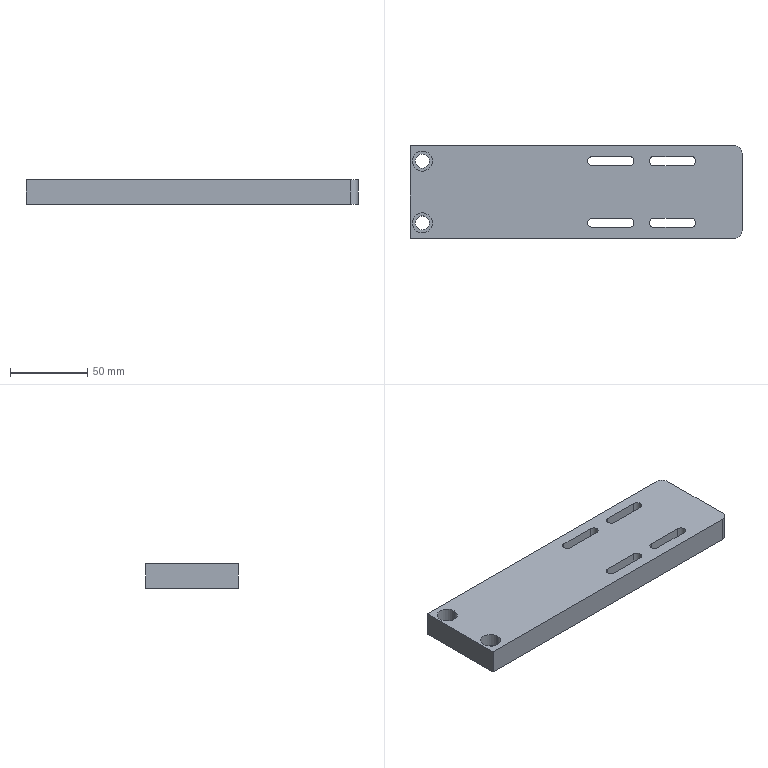NC program | Mastercam | posted with a generic post | part box 215 x 60 x 16 mm
Lines 24 to 1423 of 6620:
N230 T10 M6
N240 G0 G90 G17 G54 X-115.323 Y-40.256 A0. S7000 M3
N250 G43 H10 Z20. M8
N260 Z1.
N270 G1 Z-16.75 F600.
N280 X-115.624 Y-39.448 Z-16.868 F3000.
N290 G3 X-116.142 Y-38.642 Z-17. I-2.109 J-.785
N300 G1 X-116.424 Y-38.172
N310 X-116.706 Y-37.594
N320 X-116.919 Y-37.071
N330 X-117.071 Y-36.601
N340 X-117.179 Y-36.179
N350 X-117.254 Y-35.799
N360 X-117.347 Y-35.146
N370 X-117.4 Y-34.565
N380 X-117.429 Y-34.035
N390 X-117.443 Y-33.54
N400 X-117.45 Y-33.069
N410 X-117.451 Y-32.614
N420 X-117.449 Y-32.17
N430 X-117.444 Y-31.733
N440 X-117.439 Y-31.299
N450 X-117.433 Y-30.868
N460 X-117.426 Y-30.438
N470 X-117.419 Y-30.009
N480 X-117.412 Y-29.58
N490 X-117.405 Y-29.151
N500 X-117.397 Y-28.721
N510 X-117.39 Y-28.292
N520 X-117.382 Y-27.863
N530 X-117.374 Y-27.433
N540 X-117.367 Y-27.003
N550 X-117.359 Y-26.573
N560 X-117.352 Y-26.142
N570 X-117.344 Y-25.712
N580 X-117.336 Y-25.281
N590 X-117.329 Y-24.849
N600 X-117.321 Y-24.418
N610 X-117.313 Y-23.986
N620 X-117.305 Y-23.554
N630 X-117.298 Y-23.122
N640 X-117.29 Y-22.689
N650 X-117.282 Y-22.256
N660 X-117.275 Y-21.824
N670 X-117.267 Y-21.39
N680 X-117.259 Y-20.957
N690 X-117.252 Y-20.524
N700 X-117.244 Y-20.09
N710 X-117.236 Y-19.656
N720 X-117.228 Y-19.222
N730 X-117.221 Y-18.788
N740 X-117.213 Y-18.353
N750 X-117.205 Y-17.919
N760 X-117.197 Y-17.484
N770 X-117.19 Y-17.049
N780 X-117.182 Y-16.614
N790 X-117.174 Y-16.179
N800 X-117.166 Y-15.743
N810 X-117.159 Y-15.308
N820 X-117.151 Y-14.872
N830 X-117.143 Y-14.436
N840 X-117.135 Y-14.
N850 X-117.128 Y-13.564
N860 X-117.12 Y-13.128
N870 X-117.112 Y-12.692
N880 X-117.104 Y-12.255
N890 X-117.097 Y-11.819
N900 X-117.089 Y-11.382
N910 X-117.081 Y-10.945
N920 X-117.073 Y-10.508
N930 X-117.065 Y-10.071
N940 X-117.058 Y-9.634
N950 X-117.05 Y-9.197
N960 X-117.042 Y-8.759
N970 X-117.034 Y-8.322
N980 X-117.026 Y-7.884
N990 X-117.019 Y-7.446
N1000 X-117.011 Y-7.008
N1010 X-117.003 Y-6.571
N1020 X-116.995 Y-6.133
N1030 X-116.987 Y-5.694
N1040 X-116.98 Y-5.256
N1050 X-116.972 Y-4.818
N1060 X-116.964 Y-4.379
N1070 X-116.956 Y-3.941
N1080 X-116.948 Y-3.502
N1090 X-116.941 Y-3.064
N1100 X-116.933 Y-2.625
N1110 X-116.925 Y-2.186
N1120 X-116.917 Y-1.747
N1130 X-116.909 Y-1.308
N1140 X-116.902 Y-.869
N1150 X-116.894 Y-.43
N1160 X-116.886 Y.009
N1170 X-116.878 Y.449
N1180 X-116.87 Y.888
N1190 X-116.862 Y1.328
N1200 X-116.855 Y1.767
N1210 X-116.847 Y2.207
N1220 X-116.839 Y2.647
N1230 X-116.831 Y3.086
N1240 X-116.823 Y3.526
N1250 X-116.815 Y3.966
N1260 X-116.808 Y4.406
N1270 X-116.8 Y4.846
N1280 X-116.792 Y5.286
N1290 X-116.784 Y5.727
N1300 X-116.776 Y6.167
N1310 X-116.768 Y6.607
N1320 X-116.761 Y7.048
N1330 X-116.753 Y7.488
N1340 X-116.745 Y7.929
N1350 X-116.737 Y8.369
N1360 X-116.729 Y8.81
N1370 X-116.721 Y9.251
N1380 X-116.714 Y9.692
N1390 X-116.706 Y10.132
N1400 X-116.698 Y10.573
N1410 X-116.69 Y11.014
N1420 X-116.682 Y11.455
N1430 X-116.674 Y11.896
N1440 X-116.666 Y12.338
N1450 X-116.659 Y12.779
N1460 X-116.651 Y13.22
N1470 X-116.643 Y13.661
N1480 X-116.635 Y14.103
N1490 X-116.627 Y14.544
N1500 X-116.619 Y14.986
N1510 X-116.611 Y15.427
N1520 X-116.604 Y15.869
N1530 X-116.596 Y16.31
N1540 X-116.588 Y16.752
N1550 X-116.58 Y17.194
N1560 X-116.572 Y17.636
N1570 X-116.564 Y18.078
N1580 X-116.556 Y18.519
N1590 X-116.549 Y18.961
N1600 X-116.541 Y19.403
N1610 X-116.533 Y19.845
N1620 X-116.525 Y20.288
N1630 X-116.517 Y20.73
N1640 X-116.509 Y21.172
N1650 X-116.501 Y21.614
N1660 X-116.493 Y22.056
N1670 X-116.486 Y22.499
N1680 X-116.478 Y22.941
N1690 X-116.47 Y23.384
N1700 X-116.462 Y23.826
N1710 X-116.454 Y24.269
N1720 X-116.446 Y24.711
N1730 X-116.438 Y25.154
N1740 X-116.43 Y25.596
N1750 X-116.422 Y26.039
N1760 X-116.415 Y26.482
N1770 X-116.407 Y26.925
N1780 X-116.399 Y27.367
N1790 X-116.391 Y27.81
N1800 X-116.383 Y28.253
N1810 X-116.375 Y28.696
N1820 X-116.367 Y29.139
N1830 X-116.359 Y29.582
N1840 X-116.352 Y30.025
N1850 X-116.344 Y30.468
N1860 X-116.336 Y30.911
N1870 X-116.328 Y31.355
N1880 X-116.316 Y31.853
N1890 X-116.262 Y32.341
N1900 X-116.139 Y32.852
N1910 X-115.945 Y33.376
N1920 X-115.68 Y33.895
N1930 X-115.353 Y34.396
N1940 X-114.969 Y34.868
N1950 X-114.541 Y35.305
N1960 X-114.077 Y35.702
N1970 X-113.587 Y36.059
N1980 X-113.078 Y36.377
N1990 X-112.558 Y36.661
N2000 X-112.03 Y36.91
N2010 X-111.499 Y37.13
N2020 X-110.968 Y37.322
N2030 X-110.439 Y37.49
N2040 X-109.913 Y37.637
N2050 X-109.391 Y37.764
N2060 X-108.874 Y37.876
N2070 X-108.363 Y37.973
N2080 X-107.856 Y38.057
N2090 X-107.354 Y38.131
N2100 X-106.857 Y38.195
N2110 X-106.364 Y38.251
N2120 X-105.875 Y38.3
N2130 X-105.391 Y38.343
N2140 X-104.909 Y38.381
N2150 X-104.431 Y38.414
N2160 X-103.956 Y38.442
N2170 X-103.483 Y38.468
N2180 X-103.013 Y38.49
N2190 X-102.545 Y38.509
N2200 X-102.078 Y38.526
N2210 X-101.614 Y38.541
N2220 X-101.151 Y38.554
N2230 X-100.689 Y38.566
N2240 X-100.228 Y38.576
N2250 X-99.768 Y38.585
N2260 X-99.309 Y38.592
N2270 X-98.851 Y38.599
N2280 X-98.394 Y38.605
N2290 X-97.938 Y38.611
N2300 X-97.482 Y38.615
N2310 X-97.026 Y38.62
N2320 X-96.571 Y38.623
N2330 X-96.116 Y38.626
N2340 X-95.662 Y38.629
N2350 X-95.208 Y38.632
N2360 X-94.754 Y38.634
N2370 X-94.301 Y38.636
N2380 X-93.847 Y38.637
N2390 X-93.394 Y38.639
N2400 X-92.941 Y38.64
N2410 X-92.488 Y38.641
N2420 X-92.036 Y38.642
N2430 X-91.583 Y38.643
N2440 X-91.131 Y38.644
N2450 X-90.678 Y38.645
N2460 X-90.226
N2470 X-89.774 Y38.646
N2480 X-89.321
N2490 X-88.869 Y38.647
N2500 X-88.417
N2510 X-87.965 Y38.648
N2520 X-87.513
N2530 X-87.061
N2540 X-86.609
N2550 X-86.157 Y38.649
N2560 X-85.705
N2570 X-85.253
N2580 X-84.801
N2590 X-84.349
N2600 X-83.897
N2610 X-83.446
N2620 X-82.994
N2630 X-82.542
N2640 X-82.09 Y38.65
N2650 X-81.638
N2660 X-81.186
N2670 X-80.735
N2680 X-80.283
N2690 X-79.831
N2700 X-79.379
N2710 X-78.927
N2720 X-78.476
N2730 X-78.024
N2740 X-77.572
N2750 X-77.12
N2760 X-76.668
N2770 X-76.217
N2780 X-75.765
N2790 X-75.313
N2800 X-74.861
N2810 X-74.41
N2820 X-73.958
N2830 X-73.506
N2840 X-73.054
N2850 X-72.602
N2860 X-72.151
N2870 X-71.699
N2880 X-71.247
N2890 X-70.795
N2900 X-70.344
N2910 X-69.892
N2920 X-69.44
N2930 X-68.988
N2940 X-68.536
N2950 X-68.085
N2960 X-67.633
N2970 X-67.181
N2980 X-66.729
N2990 X-66.278
N3000 X-65.826
N3010 X-65.374
N3020 X-64.922
N3030 X-64.47
N3040 X-64.019
N3050 X-63.567
N3060 X-63.115
N3070 X-62.663
N3080 X-62.212
N3090 X-61.76
N3100 X-61.308
N3110 X-60.856
N3120 X-60.404
N3130 X-59.953
N3140 X-59.501
N3150 X-59.049
N3160 X-58.597
N3170 X-58.146
N3180 X-57.694
N3190 X-57.242
N3200 X-56.79
N3210 X-56.338
N3220 X-55.887
N3230 X-55.435
N3240 X-54.983
N3250 X-54.531
N3260 X-54.08
N3270 X-53.628
N3280 X-53.176
N3290 X-52.724
N3300 X-52.273
N3310 X-51.821
N3320 X-51.369
N3330 X-50.917
N3340 X-50.465
N3350 X-50.014
N3360 X-49.562
N3370 X-49.11
N3380 X-48.658
N3390 X-48.207
N3400 X-47.755
N3410 X-47.303
N3420 X-46.851
N3430 X-46.399
N3440 X-45.948
N3450 X-45.496
N3460 X-45.044
N3470 X-44.592
N3480 X-44.141
N3490 X-43.689
N3500 X-43.237
N3510 X-42.785
N3520 X-42.333
N3530 X-41.882
N3540 X-41.43
N3550 X-40.978
N3560 X-40.526
N3570 X-40.075
N3580 X-39.623
N3590 X-39.171
N3600 X-38.719
N3610 X-38.268
N3620 X-37.816
N3630 X-37.364
N3640 X-36.912
N3650 X-36.46
N3660 X-36.009
N3670 X-35.557
N3680 X-35.105
N3690 X-34.653
N3700 X-34.202
N3710 X-33.75
N3720 X-33.298
N3730 X-32.846
N3740 X-32.394
N3750 X-31.943
N3760 X-31.491
N3770 X-31.039
N3780 X-30.587
N3790 X-30.136
N3800 X-29.684
N3810 X-29.232
N3820 X-28.78
N3830 X-28.328
N3840 X-27.877
N3850 X-27.425
N3860 X-26.973
N3870 X-26.521
N3880 X-26.07
N3890 X-25.618
N3900 X-25.166
N3910 X-24.714
N3920 X-24.263
N3930 X-23.811
N3940 X-23.359
N3950 X-22.907
N3960 X-22.455
N3970 X-22.004
N3980 X-21.552
N3990 X-21.1
N4000 X-20.648
N4010 X-20.197
N4020 X-19.745
N4030 X-19.293
N4040 X-18.841
N4050 X-18.389
N4060 X-17.938
N4070 X-17.486
N4080 X-17.034
N4090 X-16.582
N4100 X-16.131
N4110 X-15.679
N4120 X-15.227
N4130 X-14.775
N4140 X-14.323
N4150 X-13.872
N4160 X-13.42
N4170 X-12.968
N4180 X-12.516
N4190 X-12.065
N4200 X-11.613
N4210 X-11.161
N4220 X-10.709
N4230 X-10.257
N4240 X-9.806
N4250 X-9.354
N4260 X-8.902
N4270 X-8.45
N4280 X-7.999
N4290 X-7.547
N4300 X-7.095
N4310 X-6.643
N4320 X-6.192
N4330 X-5.74
N4340 X-5.288
N4350 X-4.836
N4360 X-4.384
N4370 X-3.933
N4380 X-3.481
N4390 X-3.029
N4400 X-2.577
N4410 X-2.126
N4420 X-1.674
N4430 X-1.222
N4440 X-.77
N4450 X-.318
N4460 X.133
N4470 X.585
N4480 X1.037
N4490 X1.489
N4500 X1.94
N4510 X2.392
N4520 X2.844
N4530 X3.296
N4540 X3.748
N4550 X4.199
N4560 X4.651
N4570 X5.103
N4580 X5.555
N4590 X6.006
N4600 X6.458
N4610 X6.91
N4620 X7.362
N4630 X7.813
N4640 X8.265
N4650 X8.717
N4660 X9.169
N4670 X9.621
N4680 X10.072
N4690 X10.524
N4700 X10.976
N4710 X11.428
N4720 X11.879
N4730 X12.331
N4740 X12.783
N4750 X13.235
N4760 X13.687
N4770 X14.138
N4780 X14.59
N4790 X15.042
N4800 X15.494
N4810 X15.945
N4820 X16.397
N4830 X16.849
N4840 X17.301
N4850 X17.753
N4860 X18.204
N4870 X18.656
N4880 X19.108
N4890 X19.56
N4900 X20.011
N4910 X20.463
N4920 X20.915
N4930 X21.367
N4940 X21.818
N4950 X22.27
N4960 X22.722
N4970 X23.174
N4980 X23.626
N4990 X24.077
N5000 X24.529
N5010 X24.981
N5020 X25.433
N5030 X25.884
N5040 X26.336
N5050 X26.788
N5060 X27.24
N5070 X27.692
N5080 X28.143
N5090 X28.595
N5100 X29.047
N5110 X29.499
N5120 X29.95
N5130 X30.402
N5140 X30.854
N5150 X31.306
N5160 X31.758
N5170 X32.209
N5180 X32.661
N5190 X33.113
N5200 X33.565
N5210 X34.016
N5220 X34.468
N5230 X34.92
N5240 X35.372
N5250 X35.823
N5260 X36.275
N5270 X36.727
N5280 X37.179
N5290 X37.631
N5300 X38.082
N5310 X38.534
N5320 X38.986
N5330 X39.438
N5340 X39.889
N5350 X40.341
N5360 X40.793
N5370 X41.245
N5380 X41.697
N5390 X42.148
N5400 X42.6
N5410 X43.052
N5420 X43.504
N5430 X43.955
N5440 X44.407
N5450 X44.859
N5460 X45.311
N5470 X45.763
N5480 X46.214
N5490 X46.666
N5500 X47.118
N5510 X47.57
N5520 X48.021
N5530 X48.473
N5540 X48.925
N5550 X49.377
N5560 X49.828
N5570 X50.28
N5580 X50.732
N5590 X51.184
N5600 X51.636
N5610 X52.087
N5620 X52.539
N5630 X52.991
N5640 X53.443
N5650 X53.894
N5660 X54.346
N5670 X54.798
N5680 X55.25
N5690 X55.702
N5700 X56.153
N5710 X56.605
N5720 X57.057
N5730 X57.509
N5740 X57.96
N5750 X58.412
N5760 X58.864
N5770 X59.316
N5780 X59.768
N5790 X60.219
N5800 X60.671
N5810 X61.123
N5820 X61.575
N5830 X62.026
N5840 X62.478
N5850 X62.93
N5860 X63.382
N5870 X63.833
N5880 X64.285
N5890 X64.737
N5900 X65.189
N5910 X65.641
N5920 X66.092
N5930 X66.544
N5940 X66.996
N5950 X67.448
N5960 X67.899
N5970 X68.351
N5980 X68.803
N5990 X69.255
N6000 X69.707
N6010 X70.158
N6020 X70.61
N6030 X71.062
N6040 X71.514
N6050 X71.965
N6060 X72.417
N6070 X72.869
N6080 X73.321
N6090 X73.773
N6100 X74.224
N6110 X74.676
N6120 X75.128
N6130 X75.58
N6140 X76.031
N6150 X76.483
N6160 X76.935
N6170 X77.387
N6180 X77.838
N6190 X78.29
N6200 X78.742
N6210 X79.194
N6220 X79.646
N6230 X80.097
N6240 X80.549
N6250 X81.001
N6260 X81.453
N6270 X81.904
N6280 X82.356
N6290 X82.808
N6300 X83.26
N6310 X83.712
N6320 X84.163
N6330 X84.615
N6340 X85.067
N6350 X85.519
N6360 X85.97
N6370 X86.422
N6380 X86.874
N6390 X87.326
N6400 X87.778
N6410 X88.229
N6420 X88.681
N6430 X89.133
N6440 X89.585
N6450 X90.036
N6460 X90.488
N6470 X90.94
N6480 X91.392
N6490 X91.843
N6500 X92.295
N6510 X92.747
N6520 X93.199
N6530 X93.651
N6540 X94.102
N6550 X94.554
N6560 X95.006
N6570 X95.458
N6580 X95.909
N6590 X96.361
N6600 X96.813
N6610 X97.265
N6620 X97.717
N6630 X98.168
N6640 X98.62
N6650 X99.072
N6660 X99.524
N6670 X99.975
N6680 X100.427
N6690 X100.879
N6700 X101.331
N6710 X101.783
N6720 X102.234
N6730 X102.686
N6740 X103.138
N6750 X103.59
N6760 X104.041
N6770 X104.493
N6780 X104.945
N6790 X105.397
N6800 X105.848
N6810 X106.3
N6820 X106.752
N6830 X107.204
N6840 X107.656
N6850 X108.107
N6860 X108.559
N6870 X109.026
N6880 X109.511 Y38.623
N6890 X109.991 Y38.537
N6900 X110.494 Y38.386
N6910 X111.005 Y38.166
N6920 X111.509 Y37.882
N6930 X111.995 Y37.538
N6940 X112.454 Y37.144
N6950 X112.878 Y36.708
N6960 X113.266 Y36.239
N6970 X113.616 Y35.745
N6980 X113.929 Y35.234
N6990 X114.206 Y34.712
N7000 X114.45 Y34.184
N7010 X114.665 Y33.652
N7020 X114.853 Y33.122
N7030 X115.017 Y32.593
N7040 X115.16 Y32.068
N7050 X115.285 Y31.547
N7060 X115.393 Y31.031
N7070 X115.488 Y30.52
N7080 X115.57 Y30.014
N7090 X115.642 Y29.513
N7100 X115.705 Y29.016
N7110 X115.76 Y28.525
N7120 X115.808 Y28.037
N7130 X115.85 Y27.552
N7140 X115.887 Y27.072
N7150 X115.919 Y26.594
N7160 X115.947 Y26.119
N7170 X115.972 Y25.647
N7180 X115.993 Y25.177
N7190 X116.012 Y24.709
N7200 X116.029 Y24.243
N7210 X116.043 Y23.779
N7220 X116.056 Y23.316
N7230 X116.067 Y22.854
N7240 X116.077 Y22.394
N7250 X116.086 Y21.934
N7260 X116.094 Y21.475
N7270 X116.1 Y21.018
N7280 X116.106 Y20.56
N7290 X116.112 Y20.104
N7300 X116.116 Y19.648
N7310 X116.12 Y19.193
N7320 X116.124 Y18.738
N7330 X116.127 Y18.283
N7340 X116.13 Y17.829
N7350 X116.132 Y17.375
N7360 X116.134 Y16.921
N7370 X116.136 Y16.467
N7380 X116.138 Y16.014
N7390 X116.139 Y15.561
N7400 X116.14 Y15.108
N7410 X116.142 Y14.655
N7420 X116.143 Y14.203
N7430 X116.144 Y13.75
N7440 Y13.298
N7450 X116.145 Y12.845
N7460 X116.146 Y12.393
N7470 Y11.941
N7480 X116.147 Y11.488
N7490 Y11.036
N7500 Y10.584
N7510 X116.148 Y10.132
N7520 Y9.68
N7530 Y9.228
N7540 Y8.776
N7550 X116.149 Y8.324
N7560 Y7.872
N7570 Y7.42
N7580 Y6.968
N7590 Y6.516
N7600 Y6.065
N7610 Y5.613
N7620 Y5.161
N7630 Y4.709
N7640 X116.15 Y4.257
N7650 Y3.805
N7660 Y3.354
N7670 Y2.902
N7680 Y2.45
N7690 Y1.998
N7700 Y1.546
N7710 Y1.095
N7720 Y.643
N7730 Y.191
N7740 Y-.261
N7750 Y-.713
N7760 Y-1.164
N7770 Y-1.616
N7780 Y-2.068
N7790 Y-2.52
N7800 Y-2.972
N7810 Y-3.423
N7820 Y-3.875
N7830 Y-4.327
N7840 Y-4.779
N7850 Y-5.231
N7860 Y-5.682
N7870 Y-6.134
N7880 Y-6.586
N7890 Y-7.038
N7900 Y-7.489
N7910 Y-7.941
N7920 Y-8.393
N7930 Y-8.845
N7940 Y-9.296
N7950 Y-9.748
N7960 Y-10.2
N7970 Y-10.652
N7980 Y-11.104
N7990 Y-11.555
N8000 Y-12.007
N8010 Y-12.459
N8020 Y-12.911
N8030 Y-13.362
N8040 Y-13.814
N8050 Y-14.266
N8060 Y-14.718
N8070 Y-15.17
N8080 Y-15.621
N8090 Y-16.073
N8100 Y-16.525
N8110 Y-16.977
N8120 Y-17.428
N8130 Y-17.88
N8140 Y-18.332
N8150 Y-18.784
N8160 Y-19.236
N8170 Y-19.687
N8180 Y-20.139
N8190 Y-20.591
N8200 Y-21.043
N8210 Y-21.494
N8220 Y-21.946
N8230 Y-22.398
N8240 Y-22.85
N8250 Y-23.302
N8260 Y-23.753
N8270 Y-24.205
N8280 Y-24.657
N8290 Y-25.109
N8300 Y-25.56
N8310 Y-26.012
N8320 Y-26.464
N8330 Y-26.916
N8340 Y-27.367
N8350 Y-27.819
N8360 Y-28.271
N8370 Y-28.723
N8380 Y-29.175
N8390 Y-29.626
N8400 Y-30.078
N8410 Y-30.53
N8420 Y-30.982
N8430 Y-31.433
N8440 X116.132 Y-31.93
N8450 X116.057 Y-32.404
N8460 X115.917 Y-32.904
N8470 X115.71 Y-33.415
N8480 X115.436 Y-33.921
N8490 X115.103 Y-34.411
N8500 X114.717 Y-34.875
N8510 X114.288 Y-35.306
N8520 X113.824 Y-35.701
N8530 X113.334 Y-36.057
N8540 X112.826 Y-36.376
N8550 X112.305 Y-36.659
N8560 X111.777 Y-36.909
N8570 X111.246 Y-37.129
N8580 X110.715 Y-37.321
N8590 X110.186 Y-37.489
N8600 X109.66 Y-37.636
N8610 X109.138 Y-37.764
N8620 X108.622 Y-37.875
N8630 X108.11 Y-37.972
N8640 X107.603 Y-38.057
N8650 X107.101 Y-38.13
N8660 X106.604 Y-38.195
N8670 X106.111 Y-38.251
N8680 X105.623 Y-38.3
N8690 X105.138 Y-38.343
N8700 X104.656 Y-38.381
N8710 X104.178 Y-38.413
N8720 X103.703 Y-38.442
N8730 X103.23 Y-38.467
N8740 X102.76 Y-38.49
N8750 X102.292 Y-38.509
N8760 X101.825 Y-38.526
N8770 X101.361 Y-38.541
N8780 X100.897 Y-38.554
N8790 X100.436 Y-38.566
N8800 X99.975 Y-38.576
N8810 X99.515 Y-38.585
N8820 X99.056 Y-38.592
N8830 X98.598 Y-38.599
N8840 X98.141 Y-38.605
N8850 X97.685 Y-38.611
N8860 X97.229 Y-38.615
N8870 X96.773 Y-38.62
N8880 X96.318 Y-38.623
N8890 X95.863 Y-38.626
N8900 X95.409 Y-38.629
N8910 X94.955 Y-38.632
N8920 X94.501 Y-38.634
N8930 X94.048 Y-38.636
N8940 X93.594 Y-38.637
N8950 X93.141 Y-38.639
N8960 X92.688 Y-38.64
N8970 X92.235 Y-38.641
N8980 X91.783 Y-38.642
N8990 X91.33 Y-38.643
N9000 X90.877 Y-38.644
N9010 X90.425 Y-38.645
N9020 X89.973
N9030 X89.52 Y-38.646
N9040 X89.068
N9050 X88.616 Y-38.647
N9060 X88.164
N9070 X87.712 Y-38.648
N9080 X87.26
N9090 X86.808
N9100 X86.356
N9110 X85.904 Y-38.649
N9120 X85.452
N9130 X85.
N9140 X84.548
N9150 X84.096
N9160 X83.644
N9170 X83.193
N9180 X82.741
N9190 X82.289
N9200 X81.837 Y-38.65
N9210 X81.385
N9220 X80.933
N9230 X80.482
N9240 X80.03
N9250 X79.578
N9260 X79.126
N9270 X78.674
N9280 X78.223
N9290 X77.771
N9300 X77.319
N9310 X76.867
N9320 X76.415
N9330 X75.964
N9340 X75.512
N9350 X75.06
N9360 X74.608
N9370 X74.156
N9380 X73.705
N9390 X73.253
N9400 X72.801
N9410 X72.349
N9420 X71.898
N9430 X71.446
N9440 X70.994
N9450 X70.542
N9460 X70.09
N9470 X69.639
N9480 X69.187
N9490 X68.735
N9500 X68.283
N9510 X67.832
N9520 X67.38
N9530 X66.928
N9540 X66.476
N9550 X66.024
N9560 X65.573
N9570 X65.121
N9580 X64.669
N9590 X64.217
N9600 X63.766
N9610 X63.314
N9620 X62.862
N9630 X62.41
N9640 X61.958
N9650 X61.507
N9660 X61.055
N9670 X60.603
N9680 X60.151
N9690 X59.7
N9700 X59.248
N9710 X58.796
N9720 X58.344
N9730 X57.892
N9740 X57.441
N9750 X56.989
N9760 X56.537
N9770 X56.085
N9780 X55.634
N9790 X55.182
N9800 X54.73
N9810 X54.278
N9820 X53.827
N9830 X53.375
N9840 X52.923
N9850 X52.471
N9860 X52.019
N9870 X51.568
N9880 X51.116
N9890 X50.664
N9900 X50.212
N9910 X49.761
N9920 X49.309
N9930 X48.857
N9940 X48.405
N9950 X47.953
N9960 X47.502
N9970 X47.05
N9980 X46.598
N9990 X46.146
N100 X45.695
N110 X45.243
N120 X44.791
N130 X44.339
N140 X43.887
N150 X43.436
N160 X42.984
N170 X42.532
N180 X42.08
N190 X41.629
N200 X41.177
N210 X40.725
N220 X40.273
N230 X39.822
N240 X39.37
N250 X38.918
N260 X38.466
N270 X38.014
N280 X37.563
N290 X37.111
N300 X36.659
N310 X36.207
N320 X35.756
N330 X35.304
N340 X34.852
N350 X34.4
N360 X33.948
N370 X33.497
N380 X33.045
N390 X32.593
N400 X32.141
N410 X31.69
N420 X31.238
N430 X30.786
N440 X30.334
N450 X29.882
N460 X29.431
N470 X28.979
N480 X28.527
N490 X28.075
N500 X27.624
N510 X27.172
N520 X26.72
N530 X26.268
N540 X25.817
N550 X25.365
N560 X24.913
N570 X24.461
N580 X24.009
N590 X23.558
N600 X23.106
N610 X22.654
N620 X22.202
N630 X21.751
N640 X21.299
N650 X20.847
N660 X20.395
N670 X19.943
N680 X19.492
N690 X19.04
N700 X18.588
N710 X18.136
N720 X17.685
N730 X17.233
N740 X16.781
N750 X16.329
N760 X15.877
N770 X15.426
N780 X14.974
N790 X14.522
N800 X14.07
N810 X13.619
N820 X13.167
N830 X12.715
N840 X12.263
N850 X11.812
N860 X11.36
N870 X10.908
N880 X10.456
N890 X10.004
N900 X9.553
N910 X9.101
N920 X8.649
N930 X8.197
N940 X7.746
N950 X7.294
N960 X6.842
N970 X6.39
N980 X5.938
N990 X5.487
N1000 X5.035
N1010 X4.583
N1020 X4.131
N1030 X3.68
N1040 X3.228
N1050 X2.776
N1060 X2.324
N1070 X1.872
N1080 X1.421
N1090 X.969
N1100 X.517
N1110 X.065
N1120 X-.386
N1130 X-.838
N1140 X-1.29
N1150 X-1.742
N1160 X-2.193
N1170 X-2.645
N1180 X-3.097
N1190 X-3.549
N1200 X-4.001
N1210 X-4.452
N1220 X-4.904
N1230 X-5.356
N1240 X-5.808
N1250 X-6.259
N1260 X-6.711
N1270 X-7.163
N1280 X-7.615
N1290 X-8.067
N1300 X-8.518
N1310 X-8.97
N1320 X-9.422
N1330 X-9.874
N1340 X-10.325
N1350 X-10.777
N1360 X-11.229
N1370 X-11.681
N1380 X-12.133
N1390 X-12.584
N1400 X-13.036
N1410 X-13.488
N1420 X-13.94
N1430 X-14.391
N1440 X-14.843
N1450 X-15.295
N1460 X-15.747
N1470 X-16.199
N1480 X-16.65
N1490 X-17.102
N1500 X-17.554
N1510 X-18.006
N1520 X-18.457
N1530 X-18.909
N1540 X-19.361
N1550 X-19.813
N1560 X-20.264
N1570 X-20.716
N1580 X-21.168
N1590 X-21.62
N1600 X-22.072
N1610 X-22.523
N1620 X-22.975
N1630 X-23.427
N1640 X-23.879
N1650 X-24.33
N1660 X-24.782
N1670 X-25.234
N1680 X-25.686
N1690 X-26.138
N1700 X-26.589
N1710 X-27.041
N1720 X-27.493
N1730 X-27.945
N1740 X-28.396
N1750 X-28.848
N1760 X-29.3
N1770 X-29.752
N1780 X-30.204
N1790 X-30.655
N1800 X-31.107
N1810 X-31.559
N1820 X-32.011
N1830 X-32.462
N1840 X-32.914
N1850 X-33.366
N1860 X-33.818
N1870 X-34.269
N1880 X-34.721
N1890 X-35.173
N1900 X-35.625
N1910 X-36.077
N1920 X-36.528
N1930 X-36.98
N1940 X-37.432
N1950 X-37.884
N1960 X-38.335
N1970 X-38.787
N1980 X-39.239
N1990 X-39.691
N2000 X-40.143
N2010 X-40.594
N2020 X-41.046
N2030 X-41.498
N2040 X-41.95
N2050 X-42.401
N2060 X-42.853
N2070 X-43.305
N2080 X-43.757
N2090 X-44.209
N2100 X-44.66
N2110 X-45.112
N2120 X-45.564
N2130 X-46.016
N2140 X-46.467
N2150 X-46.919
N2160 X-47.371
N2170 X-47.823
N2180 X-48.274
N2190 X-48.726
N2200 X-49.178
N2210 X-49.63
N2220 X-50.082
N2230 X-50.533
N2240 X-50.985
N2250 X-51.437
N2260 X-51.889
N2270 X-52.34
N2280 X-52.792
N2290 X-53.244
N2300 X-53.696
N2310 X-54.148
N2320 X-54.599
N2330 X-55.051
N2340 X-55.503
N2350 X-55.955
N2360 X-56.406
N2370 X-56.858
N2380 X-57.31
N2390 X-57.762
N2400 X-58.214
N2410 X-58.665
N2420 X-59.117
N2430 X-59.569
N2440 X-60.021
N2450 X-60.472
N2460 X-60.924
N2470 X-61.376
N2480 X-61.828
N2490 X-62.279
N2500 X-62.731
N2510 X-63.183
N2520 X-63.635
N2530 X-64.087
N2540 X-64.538
N2550 X-64.99
N2560 X-65.442
N2570 X-65.894
N2580 X-66.345
N2590 X-66.797
N2600 X-67.249
N2610 X-67.701
N2620 X-68.153
N2630 X-68.604
N2640 X-69.056
N2650 X-69.508
N2660 X-69.96
N2670 X-70.411
N2680 X-70.863
N2690 X-71.315
N2700 X-71.767
N2710 X-72.219
N2720 X-72.67
N2730 X-73.122
N2740 X-73.574
N2750 X-74.026
N2760 X-74.477
N2770 X-74.929
N2780 X-75.381
N2790 X-75.833
N2800 X-76.284
N2810 X-76.736
N2820 X-77.188
N2830 X-77.64
N2840 X-78.092
N2850 X-78.543
N2860 X-78.995
N2870 X-79.447
N2880 X-79.899
N2890 X-80.35
N2900 X-80.802
N2910 X-81.254
N2920 X-81.706
N2930 X-82.158
N2940 X-82.609
N2950 X-83.061
N2960 X-83.513
N2970 X-83.965
N2980 X-84.416
N2990 X-84.868
N3000 X-85.32
N3010 X-85.772
N3020 X-86.224
N3030 X-86.675
N3040 X-87.127
N3050 X-87.579
N3060 X-88.031
N3070 X-88.482
N3080 X-88.934
N3090 X-89.386
N3100 X-89.838
N3110 X-90.289
N3120 X-90.741
N3130 X-91.193
N3140 X-91.645
N3150 X-92.097
N3160 X-92.548
N3170 X-93.
N3180 X-93.452
N3190 X-93.904
N3200 X-94.355
N3210 X-94.807
N3220 X-95.259
N3230 X-95.711
N3240 X-96.163
N3250 X-96.614
N3260 X-97.066
N3270 X-97.518
N3280 X-97.97
N3290 X-98.421
N3300 X-98.873
N3310 X-99.325
N3320 X-99.777
N3330 X-100.229
N3340 X-100.68
N3350 X-101.132
N3360 X-101.584
N3370 X-102.036
N3380 X-102.487
N3390 X-102.939
N3400 X-103.391
N3410 X-103.843
N3420 X-104.294
N3430 X-104.746
N3440 X-105.198
N3450 X-105.65
N3460 X-106.102
N3470 X-106.553
N3480 X-107.005
N3490 X-107.457
N3500 X-107.909
N3510 X-108.36
N3520 X-108.822 Y-38.649
N3530 X-109.329 Y-38.606
N3540 X-109.845 Y-38.502
N3550 X-110.365 Y-38.334
N3560 X-110.881 Y-38.101
N3570 X-111.385 Y-37.806
N3580 X-111.867 Y-37.455
N3590 X-112.32 Y-37.054
N3600 X-112.739 Y-36.612
N3610 X-113.12 Y-36.138
N3620 X-113.463 Y-35.639
N3630 X-113.769 Y-35.124
N3640 X-114.039 Y-34.597
N3650 X-114.276 Y-34.065
N3660 X-114.483 Y-33.53
N3670 X-114.663 Y-32.996
N3680 X-114.819 Y-32.464
N3690 X-114.954 Y-31.936
N3700 X-115.071 Y-31.413
N3710 X-115.172 Y-30.895
N3720 X-115.258 Y-30.382
N3730 X-115.332 Y-29.874
N3740 X-115.396 Y-29.372
N3750 X-115.451 Y-28.874
N3760 X-115.498 Y-28.381
N3770 X-115.537 Y-27.892
N3780 X-115.571 Y-27.407
N3790 X-115.599 Y-26.925
N3800 X-115.623 Y-26.447
N3810 X-115.643 Y-25.971
N3820 X-115.66 Y-25.499
N3830 X-115.673 Y-25.028
N3840 X-115.684 Y-24.56
N3850 X-115.692 Y-24.093
N3860 X-115.699 Y-23.629
N3870 X-115.704 Y-23.165
N3880 X-115.707 Y-22.703
N3890 X-115.709 Y-22.243
N3900 Y-21.783
N3910 Y-21.324
N3920 X-115.707 Y-20.866
N3930 X-115.705 Y-20.409
N3940 X-115.702 Y-19.953
N3950 X-115.699 Y-19.497
N3960 X-115.695 Y-19.041
N3970 X-115.69 Y-18.586
N3980 X-115.685 Y-18.132
N3990 X-115.68 Y-17.677
N4000 X-115.674 Y-17.223
N4010 X-115.669 Y-16.77
N4020 X-115.662 Y-16.316
N4030 X-115.656 Y-15.863
N4040 X-115.649 Y-15.41
N4050 X-115.643 Y-14.957
N4060 X-115.636 Y-14.504
N4070 X-115.629 Y-14.051
N4080 X-115.621 Y-13.599
N4090 X-115.614 Y-13.146
N4100 X-115.607 Y-12.694
N4110 X-115.599 Y-12.242
N4120 X-115.592 Y-11.79
N4130 X-115.584 Y-11.337
N4140 X-115.577 Y-10.885
N4150 X-115.569 Y-10.433
N4160 X-115.561 Y-9.981
N4170 X-115.553 Y-9.529
N4180 X-115.546 Y-9.077
N4190 X-115.538 Y-8.625
N4200 X-115.53 Y-8.174
N4210 X-115.522 Y-7.722
N4220 X-115.514 Y-7.27
N4230 X-115.506 Y-6.818
N4240 X-115.498 Y-6.366
N4250 X-115.49 Y-5.914
N4260 X-115.482 Y-5.463
N4270 X-115.474 Y-5.011
N4280 X-115.467 Y-4.559
N4290 X-115.459 Y-4.107
N4300 X-115.451 Y-3.656
N4310 X-115.443 Y-3.204
N4320 X-115.435 Y-2.752